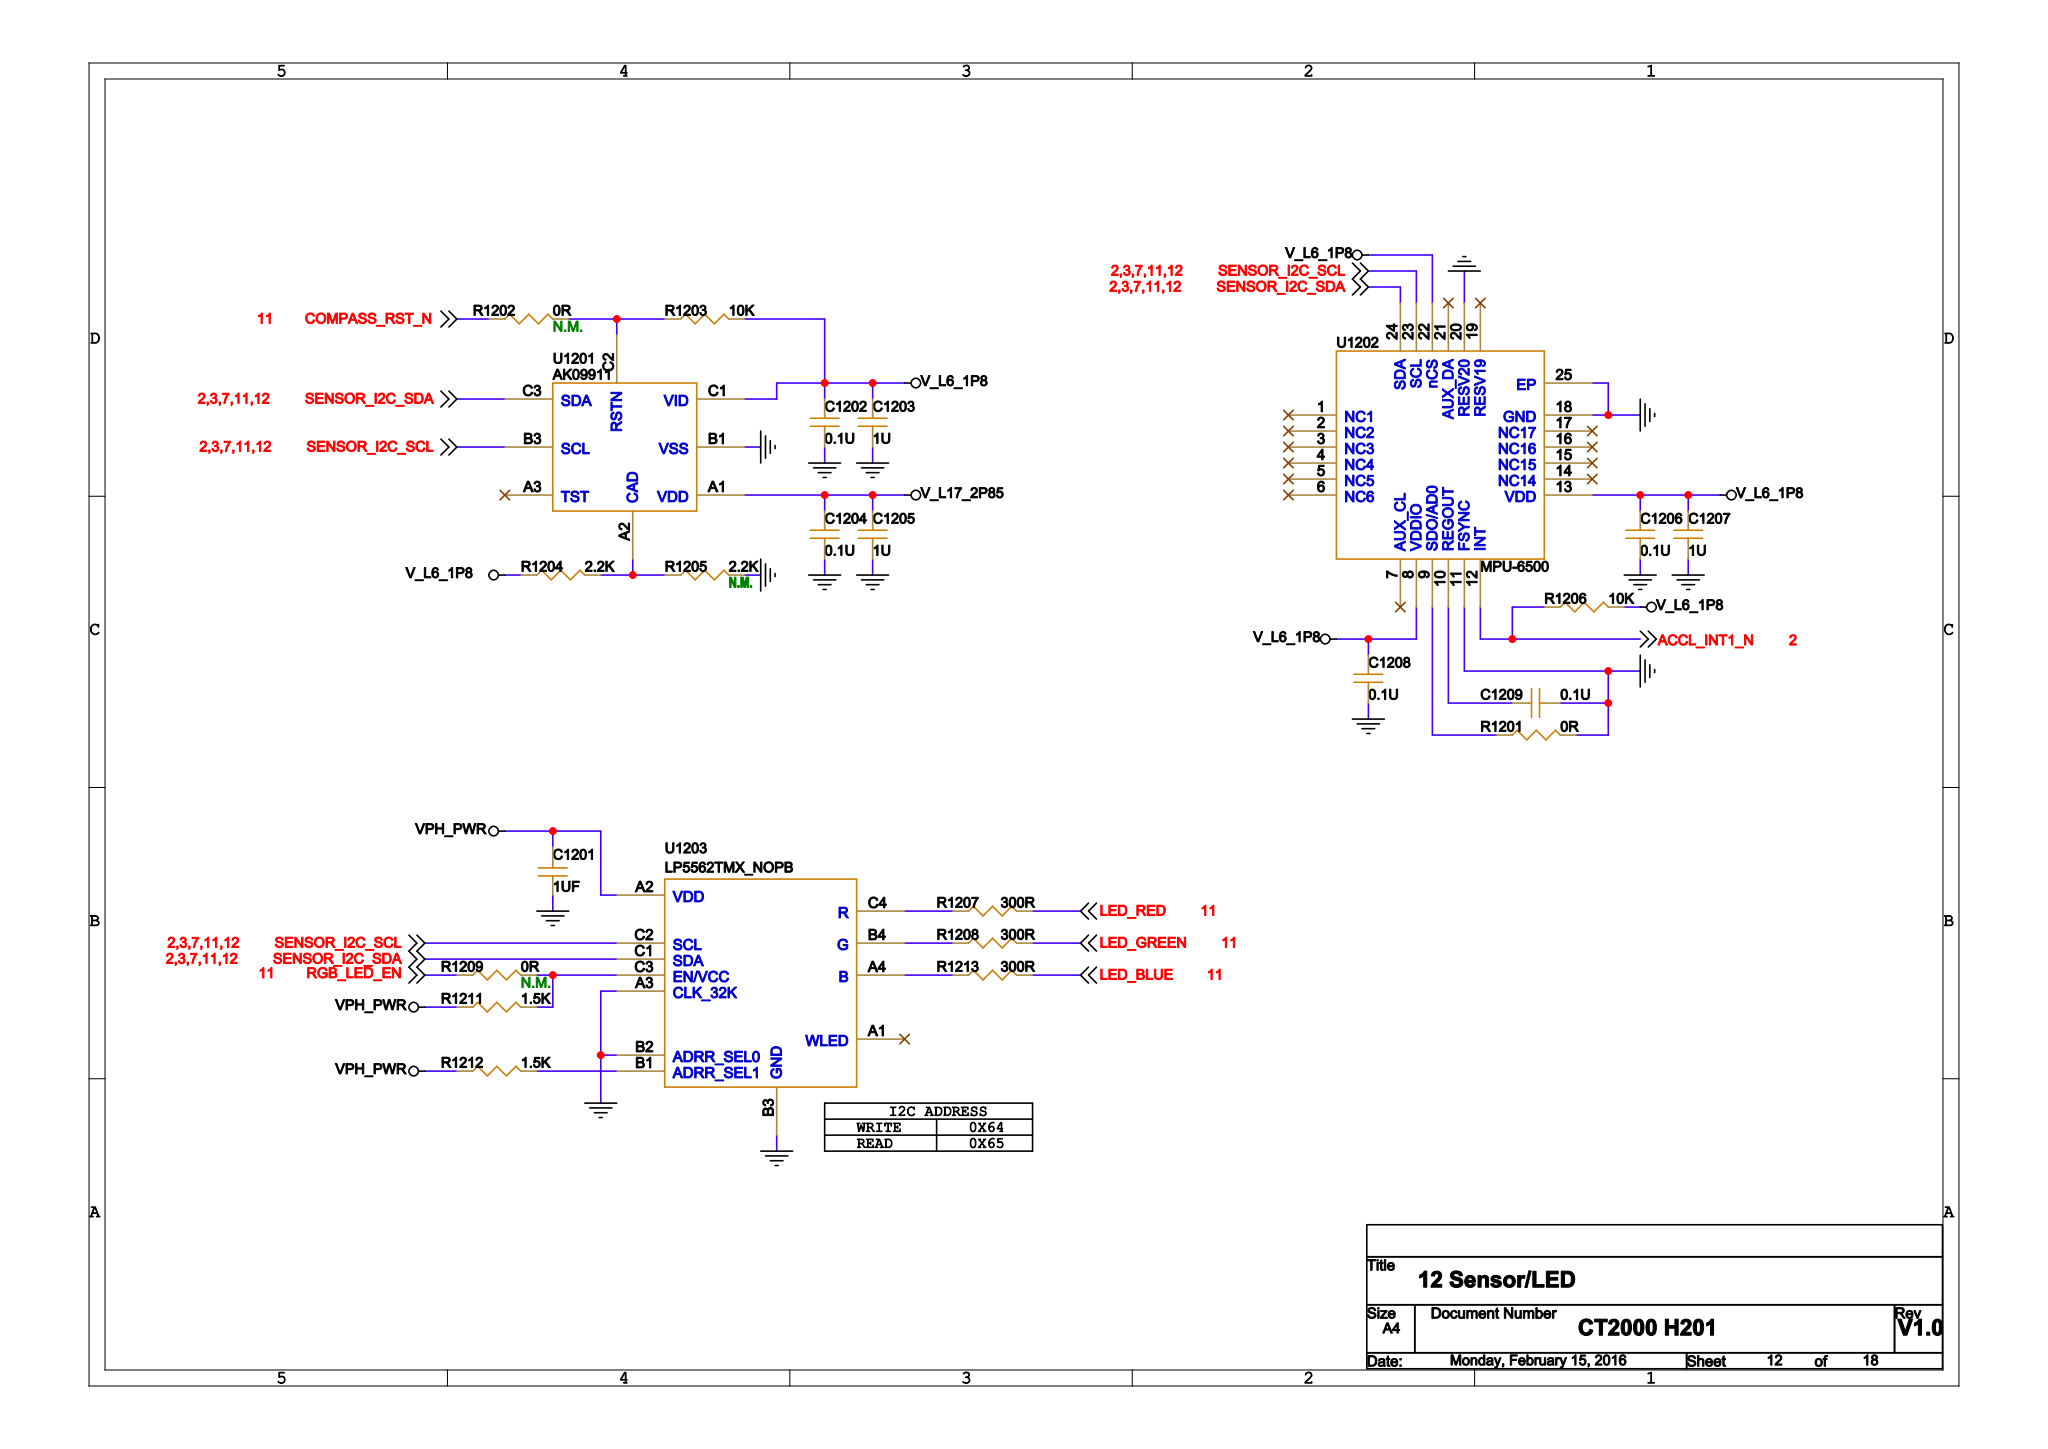Circuit board | Cadence Allegro | 573 parts | 376 nets | one sheet of the schematic
Parts on this sheet (reference | value | footprint):
C1201 | 1UF | C0402
C1202 | 0.1U | C0402
C1203 | 1U | C0402
C1204 | 0.1U | C0402
C1205 | 1U | C0402
C1206 | 0.1U | C0402
C1207 | 1U | C0402
C1208 | 0.1U | C0402
C1209 | 0.1U | C0402
R1201 | 0R | R0402
R1202 | 0R | R0402
R1203 | 10K | R0402
R1204 | 2.2K | R0402
R1205 | 2.2K | R0402
R1206 | 10K | R0402
R1207 | 300R | R0402
R1208 | 300R | R0402
R1209 | 0R | R0402
R1211 | 1.5K | R0402
R1212 | 1.5K | R0402
R1213 | 300R | R0402
U1201 | AK09911 | BGA8_1P2X1P2X0P5_0P4
U1202 | MPU-6500 | QFN24_3X3X0P9_0P4_EP
U1203 | LP5562TMX_NOPB | DSBGA12_1P218X1P618X0P775_0P4
Nets of these parts (net: part-pin ...):
GND: C1201-1 C1202-2 C1203-2 C1204-2 C1205-2 C1206-2 C1207-2 C1208-2 C1209-2 R1201-2 R1205-2 U1201-B1 U1202-11 U1202-18 U1202-20 U1202-25 U1203-A3 U1203-B2 U1203-B3
SENSOR_I2C_SDA: U1201-C3 U1202-24 U1203-C1
V_L17_2P85: C1204-1 C1205-1 U1201-A1
VPH_PWR: C1201-2 R1211-1 R1212-1 U1203-A2
SENSOR_I2C_SCL: U1201-B3 U1202-23 U1203-C2
LED_BLUE: R1213-2
LED_RED: R1207-2
LED_GREEN: R1208-2
ACCL_INT1_N: R1206-2 U1202-12
V_L6_1P8: C1202-1 C1203-1 C1206-1 C1207-1 C1208-1 R1203-2 R1204-1 R1206-1 U1201-C1 U1202-8 U1202-13 U1202-22
COMPASS_RST_N: R1202-1
RGB_LED_EN: R1209-1
N52286860: R1204-2 R1205-1 U1201-A2
N52288259: R1202-2 R1203-1 U1201-C2
N52296757: C1209-1 U1202-10
N52297477: R1201-1 U1202-9
N52738259: R1213-1 U1203-A4
N52148404: R1207-1 U1203-C4
N52148398: R1208-1 U1203-B4
N52148515: R1209-2 R1211-2 U1203-C3
N52513011: R1212-2 U1203-B1